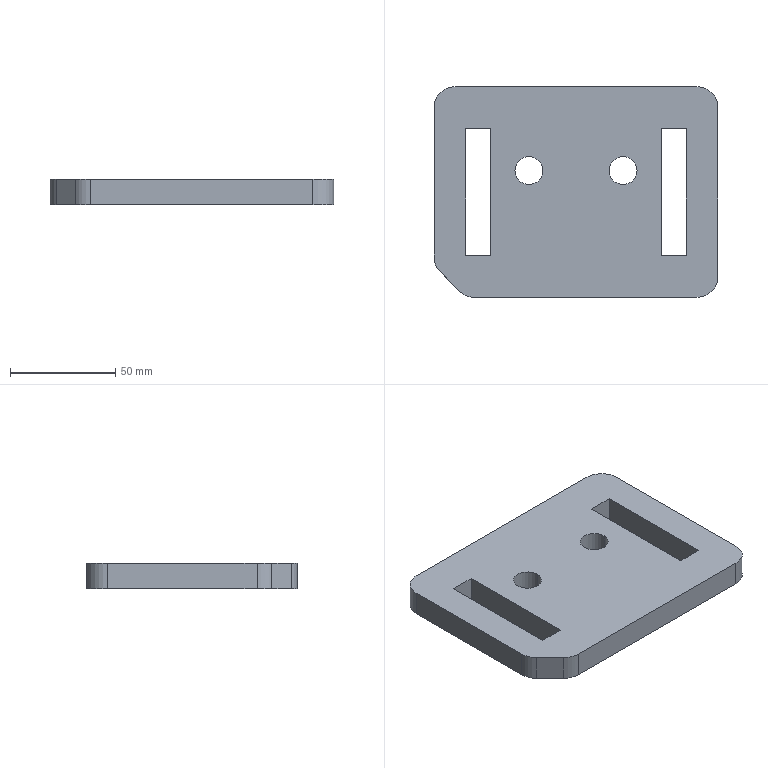Part | SolidWorks | features FlatPattern 1, SMBaseFlange 1, SheetMetal 1 | 1 solid | 24 faces | box 134.7 x 100 x 12 mm | volume 138852 mm3 | plane 15 | cylinder 9 | commonest cylinder face diameters 20 x5 13.3 x4
STEP:
#1=CARTESIAN_POINT('',(105.804,88.65,12.));
#2=VERTEX_POINT('',#1);
#3=CARTESIAN_POINT('',(119.104,88.65,12.));
#4=VERTEX_POINT('',#3);
#5=CARTESIAN_POINT('',(112.454,88.65,12.));
#6=DIRECTION('',(0.,0.,1.));
#7=DIRECTION('',(1.,0.,0.));
#8=AXIS2_PLACEMENT_3D('',#5,#6,#7);
#9=CIRCLE('',#8,6.65);
#10=EDGE_CURVE('',#2,#4,#9,.T.);
#11=ORIENTED_EDGE('',*,*,#10,.T.);
#12=CARTESIAN_POINT('',(119.104,88.65,0.));
#13=VERTEX_POINT('',#12);
#14=CARTESIAN_POINT('',(119.104,88.65,12.));
#15=DIRECTION('',(0.,0.,-1.));
#16=VECTOR('',#15,1000.);
#17=LINE('',#14,#16);
#18=EDGE_CURVE('',#4,#13,#17,.T.);
#19=ORIENTED_EDGE('',*,*,#18,.T.);
#20=CARTESIAN_POINT('',(105.804,88.65,0.));
#21=VERTEX_POINT('',#20);
#22=CARTESIAN_POINT('',(112.454,88.65,0.));
#23=DIRECTION('',(0.,0.,1.));
#24=DIRECTION('',(1.,0.,0.));
#25=AXIS2_PLACEMENT_3D('',#22,#23,#24);
#26=CIRCLE('',#25,6.65);
#27=EDGE_CURVE('',#21,#13,#26,.T.);
#28=ORIENTED_EDGE('',*,*,#27,.F.);
#29=CARTESIAN_POINT('',(105.804,88.65,12.));
#30=DIRECTION('',(0.,0.,-1.));
#31=VECTOR('',#30,1000.);
#32=LINE('',#29,#31);
#33=EDGE_CURVE('',#2,#21,#32,.T.);
#34=ORIENTED_EDGE('',*,*,#33,.F.);
#35=EDGE_LOOP('',(#11,#19,#28,#34));
#36=FACE_OUTER_BOUND('',#35,.T.);
#37=CARTESIAN_POINT('',(112.454,88.65,12.));
#38=DIRECTION('',(0.,0.,-1.));
#39=DIRECTION('',(-1.,0.,0.));
#40=AXIS2_PLACEMENT_3D('',#37,#38,#39);
#41=CYLINDRICAL_SURFACE('',#40,6.65);
#42=ADVANCED_FACE('',(#36),#41,.F.);
#43=CARTESIAN_POINT('',(61.104,88.65,12.));
#44=VERTEX_POINT('',#43);
#45=CARTESIAN_POINT('',(74.404,88.65,12.));
#46=VERTEX_POINT('',#45);
#47=CARTESIAN_POINT('',(67.754,88.65,12.));
#48=DIRECTION('',(0.,0.,1.));
#49=DIRECTION('',(1.,0.,0.));
#50=AXIS2_PLACEMENT_3D('',#47,#48,#49);
#51=CIRCLE('',#50,6.65);
#52=EDGE_CURVE('',#44,#46,#51,.T.);
#53=ORIENTED_EDGE('',*,*,#52,.T.);
#54=CARTESIAN_POINT('',(74.404,88.65,0.));
#55=VERTEX_POINT('',#54);
#56=CARTESIAN_POINT('',(74.404,88.65,12.));
#57=DIRECTION('',(0.,0.,-1.));
#58=VECTOR('',#57,1000.);
#59=LINE('',#56,#58);
#60=EDGE_CURVE('',#46,#55,#59,.T.);
#61=ORIENTED_EDGE('',*,*,#60,.T.);
#62=CARTESIAN_POINT('',(61.104,88.65,0.));
#63=VERTEX_POINT('',#62);
#64=CARTESIAN_POINT('',(67.754,88.65,0.));
#65=DIRECTION('',(0.,0.,1.));
#66=DIRECTION('',(1.,0.,0.));
#67=AXIS2_PLACEMENT_3D('',#64,#65,#66);
#68=CIRCLE('',#67,6.65);
#69=EDGE_CURVE('',#63,#55,#68,.T.);
#70=ORIENTED_EDGE('',*,*,#69,.F.);
#71=CARTESIAN_POINT('',(61.104,88.65,12.));
#72=DIRECTION('',(0.,0.,-1.));
#73=VECTOR('',#72,1000.);
#74=LINE('',#71,#73);
#75=EDGE_CURVE('',#44,#63,#74,.T.);
#76=ORIENTED_EDGE('',*,*,#75,.F.);
#77=EDGE_LOOP('',(#53,#61,#70,#76));
#78=FACE_OUTER_BOUND('',#77,.T.);
#79=CARTESIAN_POINT('',(67.754,88.65,12.));
#80=DIRECTION('',(0.,0.,-1.));
#81=DIRECTION('',(-1.,0.,0.));
#82=AXIS2_PLACEMENT_3D('',#79,#80,#81);
#83=CYLINDRICAL_SURFACE('',#82,6.65);
#84=ADVANCED_FACE('',(#78),#83,.F.);
#85=ORIENTED_EDGE('',*,*,#52,.F.);
#86=CARTESIAN_POINT('',(67.754,88.65,12.));
#87=DIRECTION('',(0.,0.,1.));
#88=DIRECTION('',(1.,0.,0.));
#89=AXIS2_PLACEMENT_3D('',#86,#87,#88);
#90=CIRCLE('',#89,6.65);
#91=EDGE_CURVE('',#46,#44,#90,.T.);
#92=ORIENTED_EDGE('',*,*,#91,.F.);
#93=EDGE_LOOP('',(#85,#92));
#94=FACE_BOUND('',#93,.T.);
#95=CARTESIAN_POINT('',(22.754,47.642,12.));
#96=VERTEX_POINT('',#95);
#97=CARTESIAN_POINT('',(25.683,40.571,12.));
#98=VERTEX_POINT('',#97);
#99=CARTESIAN_POINT('',(32.754,47.642,12.));
#100=DIRECTION('',(0.,0.,1.));
#101=DIRECTION('',(1.,0.,0.));
#102=AXIS2_PLACEMENT_3D('',#99,#100,#101);
#103=CIRCLE('',#102,10.);
#104=EDGE_CURVE('',#96,#98,#103,.T.);
#105=ORIENTED_EDGE('',*,*,#104,.T.);
#106=CARTESIAN_POINT('',(34.825,31.429,12.));
#107=VERTEX_POINT('',#106);
#108=CARTESIAN_POINT('',(34.825,31.429,12.));
#109=DIRECTION('',(0.7071,-0.7071,0.));
#110=VECTOR('',#109,1000.);
#111=LINE('',#108,#110);
#112=EDGE_CURVE('',#98,#107,#111,.T.);
#113=ORIENTED_EDGE('',*,*,#112,.T.);
#114=CARTESIAN_POINT('',(41.896,28.5,12.));
#115=VERTEX_POINT('',#114);
#116=CARTESIAN_POINT('',(41.896,38.5,12.));
#117=DIRECTION('',(0.,0.,1.));
#118=DIRECTION('',(-1.,0.,0.));
#119=AXIS2_PLACEMENT_3D('',#116,#117,#118);
#120=CIRCLE('',#119,10.);
#121=EDGE_CURVE('',#107,#115,#120,.T.);
#122=ORIENTED_EDGE('',*,*,#121,.T.);
#123=CARTESIAN_POINT('',(147.454,28.5,12.));
#124=VERTEX_POINT('',#123);
#125=CARTESIAN_POINT('',(41.896,28.5,12.));
#126=DIRECTION('',(1.,0.,0.));
#127=VECTOR('',#126,1000.);
#128=LINE('',#125,#127);
#129=EDGE_CURVE('',#115,#124,#128,.T.);
#130=ORIENTED_EDGE('',*,*,#129,.T.);
#131=CARTESIAN_POINT('',(157.454,38.5,12.));
#132=VERTEX_POINT('',#131);
#133=CARTESIAN_POINT('',(147.454,38.5,12.));
#134=DIRECTION('',(0.,0.,1.));
#135=DIRECTION('',(1.,0.,0.));
#136=AXIS2_PLACEMENT_3D('',#133,#134,#135);
#137=CIRCLE('',#136,10.);
#138=EDGE_CURVE('',#124,#132,#137,.T.);
#139=ORIENTED_EDGE('',*,*,#138,.T.);
#140=CARTESIAN_POINT('',(157.454,118.5,12.));
#141=VERTEX_POINT('',#140);
#142=CARTESIAN_POINT('',(157.454,118.5,12.));
#143=DIRECTION('',(0.,1.,0.));
#144=VECTOR('',#143,1000.);
#145=LINE('',#142,#144);
#146=EDGE_CURVE('',#132,#141,#145,.T.);
#147=ORIENTED_EDGE('',*,*,#146,.T.);
#148=CARTESIAN_POINT('',(147.454,128.5,12.));
#149=VERTEX_POINT('',#148);
#150=CARTESIAN_POINT('',(147.454,118.5,12.));
#151=DIRECTION('',(0.,0.,1.));
#152=DIRECTION('',(-1.,0.,0.));
#153=AXIS2_PLACEMENT_3D('',#150,#151,#152);
#154=CIRCLE('',#153,10.);
#155=EDGE_CURVE('',#141,#149,#154,.T.);
#156=ORIENTED_EDGE('',*,*,#155,.T.);
#157=CARTESIAN_POINT('',(32.754,128.5,12.));
#158=VERTEX_POINT('',#157);
#159=CARTESIAN_POINT('',(32.754,128.5,12.));
#160=DIRECTION('',(-1.,0.,0.));
#161=VECTOR('',#160,1000.);
#162=LINE('',#159,#161);
#163=EDGE_CURVE('',#149,#158,#162,.T.);
#164=ORIENTED_EDGE('',*,*,#163,.T.);
#165=CARTESIAN_POINT('',(22.754,118.5,12.));
#166=VERTEX_POINT('',#165);
#167=CARTESIAN_POINT('',(32.754,118.5,12.));
#168=DIRECTION('',(0.,0.,1.));
#169=DIRECTION('',(1.,0.,0.));
#170=AXIS2_PLACEMENT_3D('',#167,#168,#169);
#171=CIRCLE('',#170,10.);
#172=EDGE_CURVE('',#158,#166,#171,.T.);
#173=ORIENTED_EDGE('',*,*,#172,.T.);
#174=CARTESIAN_POINT('',(22.754,118.5,12.));
#175=DIRECTION('',(0.,-1.,0.));
#176=VECTOR('',#175,1000.);
#177=LINE('',#174,#176);
#178=EDGE_CURVE('',#166,#96,#177,.T.);
#179=ORIENTED_EDGE('',*,*,#178,.T.);
#180=EDGE_LOOP('',(#105,#113,#122,#130,#139,#147,#156,#164,#173,#179));
#181=FACE_OUTER_BOUND('',#180,.T.);
#182=ORIENTED_EDGE('',*,*,#10,.F.);
#183=CARTESIAN_POINT('',(112.454,88.65,12.));
#184=DIRECTION('',(0.,0.,1.));
#185=DIRECTION('',(1.,0.,0.));
#186=AXIS2_PLACEMENT_3D('',#183,#184,#185);
#187=CIRCLE('',#186,6.65);
#188=EDGE_CURVE('',#4,#2,#187,.T.);
#189=ORIENTED_EDGE('',*,*,#188,.F.);
#190=EDGE_LOOP('',(#182,#189));
#191=FACE_BOUND('',#190,.T.);
#192=CARTESIAN_POINT('',(142.454,108.5,12.));
#193=VERTEX_POINT('',#192);
#194=CARTESIAN_POINT('',(130.454,108.5,12.));
#195=VERTEX_POINT('',#194);
#196=CARTESIAN_POINT('',(142.454,108.5,12.));
#197=DIRECTION('',(-1.,0.,0.));
#198=VECTOR('',#197,1000.);
#199=LINE('',#196,#198);
#200=EDGE_CURVE('',#193,#195,#199,.T.);
#201=ORIENTED_EDGE('',*,*,#200,.F.);
#202=CARTESIAN_POINT('',(142.454,48.5,12.));
#203=VERTEX_POINT('',#202);
#204=CARTESIAN_POINT('',(142.454,108.5,12.));
#205=DIRECTION('',(0.,1.,0.));
#206=VECTOR('',#205,1000.);
#207=LINE('',#204,#206);
#208=EDGE_CURVE('',#203,#193,#207,.T.);
#209=ORIENTED_EDGE('',*,*,#208,.F.);
#210=CARTESIAN_POINT('',(130.454,48.5,12.));
#211=VERTEX_POINT('',#210);
#212=CARTESIAN_POINT('',(142.454,48.5,12.));
#213=DIRECTION('',(1.,0.,0.));
#214=VECTOR('',#213,1000.);
#215=LINE('',#212,#214);
#216=EDGE_CURVE('',#211,#203,#215,.T.);
#217=ORIENTED_EDGE('',*,*,#216,.F.);
#218=CARTESIAN_POINT('',(130.454,108.5,12.));
#219=DIRECTION('',(0.,-1.,0.));
#220=VECTOR('',#219,1000.);
#221=LINE('',#218,#220);
#222=EDGE_CURVE('',#195,#211,#221,.T.);
#223=ORIENTED_EDGE('',*,*,#222,.F.);
#224=EDGE_LOOP('',(#201,#209,#217,#223));
#225=FACE_BOUND('',#224,.T.);
#226=CARTESIAN_POINT('',(49.754,108.5,12.));
#227=VERTEX_POINT('',#226);
#228=CARTESIAN_POINT('',(37.754,108.5,12.));
#229=VERTEX_POINT('',#228);
#230=CARTESIAN_POINT('',(49.754,108.5,12.));
#231=DIRECTION('',(-1.,0.,0.));
#232=VECTOR('',#231,1000.);
#233=LINE('',#230,#232);
#234=EDGE_CURVE('',#227,#229,#233,.T.);
#235=ORIENTED_EDGE('',*,*,#234,.F.);
#236=CARTESIAN_POINT('',(49.754,48.5,12.));
#237=VERTEX_POINT('',#236);
#238=CARTESIAN_POINT('',(49.754,108.5,12.));
#239=DIRECTION('',(0.,1.,0.));
#240=VECTOR('',#239,1000.);
#241=LINE('',#238,#240);
#242=EDGE_CURVE('',#237,#227,#241,.T.);
#243=ORIENTED_EDGE('',*,*,#242,.F.);
#244=CARTESIAN_POINT('',(37.754,48.5,12.));
#245=VERTEX_POINT('',#244);
#246=CARTESIAN_POINT('',(49.754,48.5,12.));
#247=DIRECTION('',(1.,0.,0.));
#248=VECTOR('',#247,1000.);
#249=LINE('',#246,#248);
#250=EDGE_CURVE('',#245,#237,#249,.T.);
#251=ORIENTED_EDGE('',*,*,#250,.F.);
#252=CARTESIAN_POINT('',(37.754,108.5,12.));
#253=DIRECTION('',(0.,-1.,0.));
#254=VECTOR('',#253,1000.);
#255=LINE('',#252,#254);
#256=EDGE_CURVE('',#229,#245,#255,.T.);
#257=ORIENTED_EDGE('',*,*,#256,.F.);
#258=EDGE_LOOP('',(#235,#243,#251,#257));
#259=FACE_BOUND('',#258,.T.);
#260=CARTESIAN_POINT('',(32.754,47.642,12.));
#261=DIRECTION('',(0.,0.,1.));
#262=DIRECTION('',(1.,0.,0.));
#263=AXIS2_PLACEMENT_3D('',#260,#261,#262);
#264=PLANE('',#263);
#265=ADVANCED_FACE('',(#94,#181,#191,#225,#259),#264,.T.);
#266=CARTESIAN_POINT('',(142.454,48.5,0.));
#267=VERTEX_POINT('',#266);
#268=CARTESIAN_POINT('',(142.454,108.5,0.));
#269=VERTEX_POINT('',#268);
#270=CARTESIAN_POINT('',(142.454,108.5,0.));
#271=DIRECTION('',(0.,1.,0.));
#272=VECTOR('',#271,1000.);
#273=LINE('',#270,#272);
#274=EDGE_CURVE('',#267,#269,#273,.T.);
#275=ORIENTED_EDGE('',*,*,#274,.T.);
#276=CARTESIAN_POINT('',(130.454,108.5,0.));
#277=VERTEX_POINT('',#276);
#278=CARTESIAN_POINT('',(142.454,108.5,0.));
#279=DIRECTION('',(-1.,0.,0.));
#280=VECTOR('',#279,1000.);
#281=LINE('',#278,#280);
#282=EDGE_CURVE('',#269,#277,#281,.T.);
#283=ORIENTED_EDGE('',*,*,#282,.T.);
#284=CARTESIAN_POINT('',(130.454,48.5,0.));
#285=VERTEX_POINT('',#284);
#286=CARTESIAN_POINT('',(130.454,108.5,0.));
#287=DIRECTION('',(0.,-1.,0.));
#288=VECTOR('',#287,1000.);
#289=LINE('',#286,#288);
#290=EDGE_CURVE('',#277,#285,#289,.T.);
#291=ORIENTED_EDGE('',*,*,#290,.T.);
#292=CARTESIAN_POINT('',(142.454,48.5,0.));
#293=DIRECTION('',(1.,0.,0.));
#294=VECTOR('',#293,1000.);
#295=LINE('',#292,#294);
#296=EDGE_CURVE('',#285,#267,#295,.T.);
#297=ORIENTED_EDGE('',*,*,#296,.T.);
#298=EDGE_LOOP('',(#275,#283,#291,#297));
#299=FACE_BOUND('',#298,.T.);
#300=CARTESIAN_POINT('',(22.754,47.642,0.));
#301=VERTEX_POINT('',#300);
#302=CARTESIAN_POINT('',(25.683,40.571,0.));
#303=VERTEX_POINT('',#302);
#304=CARTESIAN_POINT('',(32.754,47.642,0.));
#305=DIRECTION('',(0.,0.,1.));
#306=DIRECTION('',(1.,0.,0.));
#307=AXIS2_PLACEMENT_3D('',#304,#305,#306);
#308=CIRCLE('',#307,10.);
#309=EDGE_CURVE('',#301,#303,#308,.T.);
#310=ORIENTED_EDGE('',*,*,#309,.F.);
#311=CARTESIAN_POINT('',(22.754,118.5,0.));
#312=VERTEX_POINT('',#311);
#313=CARTESIAN_POINT('',(22.754,118.5,0.));
#314=DIRECTION('',(0.,-1.,0.));
#315=VECTOR('',#314,1000.);
#316=LINE('',#313,#315);
#317=EDGE_CURVE('',#312,#301,#316,.T.);
#318=ORIENTED_EDGE('',*,*,#317,.F.);
#319=CARTESIAN_POINT('',(32.754,128.5,0.));
#320=VERTEX_POINT('',#319);
#321=CARTESIAN_POINT('',(32.754,118.5,0.));
#322=DIRECTION('',(0.,0.,1.));
#323=DIRECTION('',(1.,0.,0.));
#324=AXIS2_PLACEMENT_3D('',#321,#322,#323);
#325=CIRCLE('',#324,10.);
#326=EDGE_CURVE('',#320,#312,#325,.T.);
#327=ORIENTED_EDGE('',*,*,#326,.F.);
#328=CARTESIAN_POINT('',(147.454,128.5,0.));
#329=VERTEX_POINT('',#328);
#330=CARTESIAN_POINT('',(32.754,128.5,0.));
#331=DIRECTION('',(-1.,0.,0.));
#332=VECTOR('',#331,1000.);
#333=LINE('',#330,#332);
#334=EDGE_CURVE('',#329,#320,#333,.T.);
#335=ORIENTED_EDGE('',*,*,#334,.F.);
#336=CARTESIAN_POINT('',(157.454,118.5,0.));
#337=VERTEX_POINT('',#336);
#338=CARTESIAN_POINT('',(147.454,118.5,0.));
#339=DIRECTION('',(0.,0.,1.));
#340=DIRECTION('',(-1.,0.,0.));
#341=AXIS2_PLACEMENT_3D('',#338,#339,#340);
#342=CIRCLE('',#341,10.);
#343=EDGE_CURVE('',#337,#329,#342,.T.);
#344=ORIENTED_EDGE('',*,*,#343,.F.);
#345=CARTESIAN_POINT('',(157.454,38.5,0.));
#346=VERTEX_POINT('',#345);
#347=CARTESIAN_POINT('',(157.454,118.5,0.));
#348=DIRECTION('',(0.,1.,0.));
#349=VECTOR('',#348,1000.);
#350=LINE('',#347,#349);
#351=EDGE_CURVE('',#346,#337,#350,.T.);
#352=ORIENTED_EDGE('',*,*,#351,.F.);
#353=CARTESIAN_POINT('',(147.454,28.5,0.));
#354=VERTEX_POINT('',#353);
#355=CARTESIAN_POINT('',(147.454,38.5,0.));
#356=DIRECTION('',(0.,0.,1.));
#357=DIRECTION('',(1.,0.,0.));
#358=AXIS2_PLACEMENT_3D('',#355,#356,#357);
#359=CIRCLE('',#358,10.);
#360=EDGE_CURVE('',#354,#346,#359,.T.);
#361=ORIENTED_EDGE('',*,*,#360,.F.);
#362=CARTESIAN_POINT('',(41.896,28.5,0.));
#363=VERTEX_POINT('',#362);
#364=CARTESIAN_POINT('',(41.896,28.5,0.));
#365=DIRECTION('',(1.,0.,0.));
#366=VECTOR('',#365,1000.);
#367=LINE('',#364,#366);
#368=EDGE_CURVE('',#363,#354,#367,.T.);
#369=ORIENTED_EDGE('',*,*,#368,.F.);
#370=CARTESIAN_POINT('',(34.825,31.429,0.));
#371=VERTEX_POINT('',#370);
#372=CARTESIAN_POINT('',(41.896,38.5,0.));
#373=DIRECTION('',(0.,0.,1.));
#374=DIRECTION('',(-1.,0.,0.));
#375=AXIS2_PLACEMENT_3D('',#372,#373,#374);
#376=CIRCLE('',#375,10.);
#377=EDGE_CURVE('',#371,#363,#376,.T.);
#378=ORIENTED_EDGE('',*,*,#377,.F.);
#379=CARTESIAN_POINT('',(34.825,31.429,0.));
#380=DIRECTION('',(0.7071,-0.7071,0.));
#381=VECTOR('',#380,1000.);
#382=LINE('',#379,#381);
#383=EDGE_CURVE('',#303,#371,#382,.T.);
#384=ORIENTED_EDGE('',*,*,#383,.F.);
#385=EDGE_LOOP('',(#310,#318,#327,#335,#344,#352,#361,#369,#378,#384));
#386=FACE_OUTER_BOUND('',#385,.T.);
#387=ORIENTED_EDGE('',*,*,#69,.T.);
#388=CARTESIAN_POINT('',(67.754,88.65,0.));
#389=DIRECTION('',(0.,0.,1.));
#390=DIRECTION('',(1.,0.,0.));
#391=AXIS2_PLACEMENT_3D('',#388,#389,#390);
#392=CIRCLE('',#391,6.65);
#393=EDGE_CURVE('',#55,#63,#392,.T.);
#394=ORIENTED_EDGE('',*,*,#393,.T.);
#395=EDGE_LOOP('',(#387,#394));
#396=FACE_BOUND('',#395,.T.);
#397=ORIENTED_EDGE('',*,*,#27,.T.);
#398=CARTESIAN_POINT('',(112.454,88.65,0.));
#399=DIRECTION('',(0.,0.,1.));
#400=DIRECTION('',(1.,0.,0.));
#401=AXIS2_PLACEMENT_3D('',#398,#399,#400);
#402=CIRCLE('',#401,6.65);
#403=EDGE_CURVE('',#13,#21,#402,.T.);
#404=ORIENTED_EDGE('',*,*,#403,.T.);
#405=EDGE_LOOP('',(#397,#404));
#406=FACE_BOUND('',#405,.T.);
#407=CARTESIAN_POINT('',(49.754,48.5,0.));
#408=VERTEX_POINT('',#407);
#409=CARTESIAN_POINT('',(49.754,108.5,0.));
#410=VERTEX_POINT('',#409);
#411=CARTESIAN_POINT('',(49.754,108.5,0.));
#412=DIRECTION('',(0.,1.,0.));
#413=VECTOR('',#412,1000.);
#414=LINE('',#411,#413);
#415=EDGE_CURVE('',#408,#410,#414,.T.);
#416=ORIENTED_EDGE('',*,*,#415,.T.);
#417=CARTESIAN_POINT('',(37.754,108.5,0.));
#418=VERTEX_POINT('',#417);
#419=CARTESIAN_POINT('',(49.754,108.5,0.));
#420=DIRECTION('',(-1.,0.,0.));
#421=VECTOR('',#420,1000.);
#422=LINE('',#419,#421);
#423=EDGE_CURVE('',#410,#418,#422,.T.);
#424=ORIENTED_EDGE('',*,*,#423,.T.);
#425=CARTESIAN_POINT('',(37.754,48.5,0.));
#426=VERTEX_POINT('',#425);
#427=CARTESIAN_POINT('',(37.754,108.5,0.));
#428=DIRECTION('',(0.,-1.,0.));
#429=VECTOR('',#428,1000.);
#430=LINE('',#427,#429);
#431=EDGE_CURVE('',#418,#426,#430,.T.);
#432=ORIENTED_EDGE('',*,*,#431,.T.);
#433=CARTESIAN_POINT('',(49.754,48.5,0.));
#434=DIRECTION('',(1.,0.,0.));
#435=VECTOR('',#434,1000.);
#436=LINE('',#433,#435);
#437=EDGE_CURVE('',#426,#408,#436,.T.);
#438=ORIENTED_EDGE('',*,*,#437,.T.);
#439=EDGE_LOOP('',(#416,#424,#432,#438));
#440=FACE_BOUND('',#439,.T.);
#441=CARTESIAN_POINT('',(32.754,47.642,0.));
#442=DIRECTION('',(0.,0.,1.));
#443=DIRECTION('',(1.,0.,0.));
#444=AXIS2_PLACEMENT_3D('',#441,#442,#443);
#445=PLANE('',#444);
#446=ADVANCED_FACE('',(#299,#386,#396,#406,#440),#445,.F.);
#447=ORIENTED_EDGE('',*,*,#309,.T.);
#448=CARTESIAN_POINT('',(25.683,40.571,12.));
#449=DIRECTION('',(0.,0.,-1.));
#450=VECTOR('',#449,1000.);
#451=LINE('',#448,#450);
#452=EDGE_CURVE('',#98,#303,#451,.T.);
#453=ORIENTED_EDGE('',*,*,#452,.F.);
#454=ORIENTED_EDGE('',*,*,#104,.F.);
#455=CARTESIAN_POINT('',(22.754,47.642,12.));
#456=DIRECTION('',(0.,0.,-1.));
#457=VECTOR('',#456,1000.);
#458=LINE('',#455,#457);
#459=EDGE_CURVE('',#96,#301,#458,.T.);
#460=ORIENTED_EDGE('',*,*,#459,.T.);
#461=EDGE_LOOP('',(#447,#453,#454,#460));
#462=FACE_OUTER_BOUND('',#461,.T.);
#463=CARTESIAN_POINT('',(32.754,47.642,12.));
#464=DIRECTION('',(0.,0.,-1.));
#465=DIRECTION('',(-1.,0.,0.));
#466=AXIS2_PLACEMENT_3D('',#463,#464,#465);
#467=CYLINDRICAL_SURFACE('',#466,10.);
#468=ADVANCED_FACE('',(#462),#467,.T.);
#469=ORIENTED_EDGE('',*,*,#383,.T.);
#470=CARTESIAN_POINT('',(34.825,31.429,12.));
#471=DIRECTION('',(0.,0.,-1.));
#472=VECTOR('',#471,1000.);
#473=LINE('',#470,#472);
#474=EDGE_CURVE('',#107,#371,#473,.T.);
#475=ORIENTED_EDGE('',*,*,#474,.F.);
#476=ORIENTED_EDGE('',*,*,#112,.F.);
#477=ORIENTED_EDGE('',*,*,#452,.T.);
#478=EDGE_LOOP('',(#469,#475,#476,#477));
#479=FACE_OUTER_BOUND('',#478,.T.);
#480=CARTESIAN_POINT('',(34.825,31.429,12.));
#481=DIRECTION('',(0.7071,0.7071,0.));
#482=DIRECTION('',(-0.7071,0.7071,0.));
#483=AXIS2_PLACEMENT_3D('',#480,#481,#482);
#484=PLANE('',#483);
#485=ADVANCED_FACE('',(#479),#484,.F.);
#486=ORIENTED_EDGE('',*,*,#377,.T.);
#487=CARTESIAN_POINT('',(41.896,28.5,12.));
#488=DIRECTION('',(0.,0.,-1.));
#489=VECTOR('',#488,1000.);
#490=LINE('',#487,#489);
#491=EDGE_CURVE('',#115,#363,#490,.T.);
#492=ORIENTED_EDGE('',*,*,#491,.F.);
#493=ORIENTED_EDGE('',*,*,#121,.F.);
#494=ORIENTED_EDGE('',*,*,#474,.T.);
#495=EDGE_LOOP('',(#486,#492,#493,#494));
#496=FACE_OUTER_BOUND('',#495,.T.);
#497=CARTESIAN_POINT('',(41.896,38.5,12.));
#498=DIRECTION('',(0.,0.,-1.));
#499=DIRECTION('',(-1.,0.,0.));
#500=AXIS2_PLACEMENT_3D('',#497,#498,#499);
#501=CYLINDRICAL_SURFACE('',#500,10.);
#502=ADVANCED_FACE('',(#496),#501,.T.);
#503=ORIENTED_EDGE('',*,*,#368,.T.);
#504=CARTESIAN_POINT('',(147.454,28.5,12.));
#505=DIRECTION('',(0.,0.,-1.));
#506=VECTOR('',#505,1000.);
#507=LINE('',#504,#506);
#508=EDGE_CURVE('',#124,#354,#507,.T.);
#509=ORIENTED_EDGE('',*,*,#508,.F.);
#510=ORIENTED_EDGE('',*,*,#129,.F.);
#511=ORIENTED_EDGE('',*,*,#491,.T.);
#512=EDGE_LOOP('',(#503,#509,#510,#511));
#513=FACE_OUTER_BOUND('',#512,.T.);
#514=CARTESIAN_POINT('',(41.896,28.5,12.));
#515=DIRECTION('',(0.,1.,0.));
#516=DIRECTION('',(-1.,0.,0.));
#517=AXIS2_PLACEMENT_3D('',#514,#515,#516);
#518=PLANE('',#517);
#519=ADVANCED_FACE('',(#513),#518,.F.);
#520=ORIENTED_EDGE('',*,*,#360,.T.);
#521=CARTESIAN_POINT('',(157.454,38.5,12.));
#522=DIRECTION('',(0.,0.,-1.));
#523=VECTOR('',#522,1000.);
#524=LINE('',#521,#523);
#525=EDGE_CURVE('',#132,#346,#524,.T.);
#526=ORIENTED_EDGE('',*,*,#525,.F.);
#527=ORIENTED_EDGE('',*,*,#138,.F.);
#528=ORIENTED_EDGE('',*,*,#508,.T.);
#529=EDGE_LOOP('',(#520,#526,#527,#528));
#530=FACE_OUTER_BOUND('',#529,.T.);
#531=CARTESIAN_POINT('',(147.454,38.5,12.));
#532=DIRECTION('',(0.,0.,-1.));
#533=DIRECTION('',(-1.,0.,0.));
#534=AXIS2_PLACEMENT_3D('',#531,#532,#533);
#535=CYLINDRICAL_SURFACE('',#534,10.);
#536=ADVANCED_FACE('',(#530),#535,.T.);
#537=ORIENTED_EDGE('',*,*,#351,.T.);
#538=CARTESIAN_POINT('',(157.454,118.5,12.));
#539=DIRECTION('',(0.,0.,-1.));
#540=VECTOR('',#539,1000.);
#541=LINE('',#538,#540);
#542=EDGE_CURVE('',#141,#337,#541,.T.);
#543=ORIENTED_EDGE('',*,*,#542,.F.);
#544=ORIENTED_EDGE('',*,*,#146,.F.);
#545=ORIENTED_EDGE('',*,*,#525,.T.);
#546=EDGE_LOOP('',(#537,#543,#544,#545));
#547=FACE_OUTER_BOUND('',#546,.T.);
#548=CARTESIAN_POINT('',(157.454,118.5,12.));
#549=DIRECTION('',(-1.,0.,0.));
#550=DIRECTION('',(0.,0.,1.));
#551=AXIS2_PLACEMENT_3D('',#548,#549,#550);
#552=PLANE('',#551);
#553=ADVANCED_FACE('',(#547),#552,.F.);
#554=ORIENTED_EDGE('',*,*,#343,.T.);
#555=CARTESIAN_POINT('',(147.454,128.5,12.));
#556=DIRECTION('',(0.,0.,-1.));
#557=VECTOR('',#556,1000.);
#558=LINE('',#555,#557);
#559=EDGE_CURVE('',#149,#329,#558,.T.);
#560=ORIENTED_EDGE('',*,*,#559,.F.);
#561=ORIENTED_EDGE('',*,*,#155,.F.);
#562=ORIENTED_EDGE('',*,*,#542,.T.);
#563=EDGE_LOOP('',(#554,#560,#561,#562));
#564=FACE_OUTER_BOUND('',#563,.T.);
#565=CARTESIAN_POINT('',(147.454,118.5,12.));
#566=DIRECTION('',(0.,0.,-1.));
#567=DIRECTION('',(-1.,0.,0.));
#568=AXIS2_PLACEMENT_3D('',#565,#566,#567);
#569=CYLINDRICAL_SURFACE('',#568,10.);
#570=ADVANCED_FACE('',(#564),#569,.T.);
#571=ORIENTED_EDGE('',*,*,#334,.T.);
#572=CARTESIAN_POINT('',(32.754,128.5,12.));
#573=DIRECTION('',(0.,0.,-1.));
#574=VECTOR('',#573,1000.);
#575=LINE('',#572,#574);
#576=EDGE_CURVE('',#158,#320,#575,.T.);
#577=ORIENTED_EDGE('',*,*,#576,.F.);
#578=ORIENTED_EDGE('',*,*,#163,.F.);
#579=ORIENTED_EDGE('',*,*,#559,.T.);
#580=EDGE_LOOP('',(#571,#577,#578,#579));
#581=FACE_OUTER_BOUND('',#580,.T.);
#582=CARTESIAN_POINT('',(32.754,128.5,12.));
#583=DIRECTION('',(0.,-1.,0.));
#584=DIRECTION('',(0.,0.,-1.));
#585=AXIS2_PLACEMENT_3D('',#582,#583,#584);
#586=PLANE('',#585);
#587=ADVANCED_FACE('',(#581),#586,.F.);
#588=ORIENTED_EDGE('',*,*,#326,.T.);
#589=CARTESIAN_POINT('',(22.754,118.5,12.));
#590=DIRECTION('',(0.,0.,-1.));
#591=VECTOR('',#590,1000.);
#592=LINE('',#589,#591);
#593=EDGE_CURVE('',#166,#312,#592,.T.);
#594=ORIENTED_EDGE('',*,*,#593,.F.);
#595=ORIENTED_EDGE('',*,*,#172,.F.);
#596=ORIENTED_EDGE('',*,*,#576,.T.);
#597=EDGE_LOOP('',(#588,#594,#595,#596));
#598=FACE_OUTER_BOUND('',#597,.T.);
#599=CARTESIAN_POINT('',(32.754,118.5,12.));
#600=DIRECTION('',(0.,0.,-1.));
#601=DIRECTION('',(-1.,0.,0.));
#602=AXIS2_PLACEMENT_3D('',#599,#600,#601);
#603=CYLINDRICAL_SURFACE('',#602,10.);
#604=ADVANCED_FACE('',(#598),#603,.T.);
#605=ORIENTED_EDGE('',*,*,#317,.T.);
#606=ORIENTED_EDGE('',*,*,#459,.F.);
#607=ORIENTED_EDGE('',*,*,#178,.F.);
#608=ORIENTED_EDGE('',*,*,#593,.T.);
#609=EDGE_LOOP('',(#605,#606,#607,#608));
#610=FACE_OUTER_BOUND('',#609,.T.);
#611=CARTESIAN_POINT('',(22.754,118.5,12.));
#612=DIRECTION('',(1.,0.,0.));
#613=DIRECTION('',(0.,1.,0.));
#614=AXIS2_PLACEMENT_3D('',#611,#612,#613);
#615=PLANE('',#614);
#616=ADVANCED_FACE('',(#610),#615,.F.);
#617=ORIENTED_EDGE('',*,*,#60,.F.);
#618=ORIENTED_EDGE('',*,*,#91,.T.);
#619=ORIENTED_EDGE('',*,*,#75,.T.);
#620=ORIENTED_EDGE('',*,*,#393,.F.);
#621=EDGE_LOOP('',(#617,#618,#619,#620));
#622=FACE_OUTER_BOUND('',#621,.T.);
#623=CARTESIAN_POINT('',(67.754,88.65,12.));
#624=DIRECTION('',(0.,0.,-1.));
#625=DIRECTION('',(-1.,0.,0.));
#626=AXIS2_PLACEMENT_3D('',#623,#624,#625);
#627=CYLINDRICAL_SURFACE('',#626,6.65);
#628=ADVANCED_FACE('',(#622),#627,.F.);
#629=ORIENTED_EDGE('',*,*,#18,.F.);
#630=ORIENTED_EDGE('',*,*,#188,.T.);
#631=ORIENTED_EDGE('',*,*,#33,.T.);
#632=ORIENTED_EDGE('',*,*,#403,.F.);
#633=EDGE_LOOP('',(#629,#630,#631,#632));
#634=FACE_OUTER_BOUND('',#633,.T.);
#635=CARTESIAN_POINT('',(112.454,88.65,12.));
#636=DIRECTION('',(0.,0.,-1.));
#637=DIRECTION('',(-1.,0.,0.));
#638=AXIS2_PLACEMENT_3D('',#635,#636,#637);
#639=CYLINDRICAL_SURFACE('',#638,6.65);
#640=ADVANCED_FACE('',(#634),#639,.F.);
#641=ORIENTED_EDGE('',*,*,#274,.F.);
#642=CARTESIAN_POINT('',(142.454,48.5,12.));
#643=DIRECTION('',(0.,0.,-1.));
#644=VECTOR('',#643,1000.);
#645=LINE('',#642,#644);
#646=EDGE_CURVE('',#203,#267,#645,.T.);
#647=ORIENTED_EDGE('',*,*,#646,.F.);
#648=ORIENTED_EDGE('',*,*,#208,.T.);
#649=CARTESIAN_POINT('',(142.454,108.5,12.));
#650=DIRECTION('',(0.,0.,-1.));
#651=VECTOR('',#650,1000.);
#652=LINE('',#649,#651);
#653=EDGE_CURVE('',#193,#269,#652,.T.);
#654=ORIENTED_EDGE('',*,*,#653,.T.);
#655=EDGE_LOOP('',(#641,#647,#648,#654));
#656=FACE_OUTER_BOUND('',#655,.T.);
#657=CARTESIAN_POINT('',(142.454,108.5,12.));
#658=DIRECTION('',(-1.,0.,0.));
#659=DIRECTION('',(0.,0.,1.));
#660=AXIS2_PLACEMENT_3D('',#657,#658,#659);
#661=PLANE('',#660);
#662=ADVANCED_FACE('',(#656),#661,.T.);
#663=ORIENTED_EDGE('',*,*,#282,.F.);
#664=ORIENTED_EDGE('',*,*,#653,.F.);
#665=ORIENTED_EDGE('',*,*,#200,.T.);
#666=CARTESIAN_POINT('',(130.454,108.5,12.));
#667=DIRECTION('',(0.,0.,-1.));
#668=VECTOR('',#667,1000.);
#669=LINE('',#666,#668);
#670=EDGE_CURVE('',#195,#277,#669,.T.);
#671=ORIENTED_EDGE('',*,*,#670,.T.);
#672=EDGE_LOOP('',(#663,#664,#665,#671));
#673=FACE_OUTER_BOUND('',#672,.T.);
#674=CARTESIAN_POINT('',(142.454,108.5,12.));
#675=DIRECTION('',(0.,-1.,0.));
#676=DIRECTION('',(0.,0.,-1.));
#677=AXIS2_PLACEMENT_3D('',#674,#675,#676);
#678=PLANE('',#677);
#679=ADVANCED_FACE('',(#673),#678,.T.);
#680=ORIENTED_EDGE('',*,*,#290,.F.);
#681=ORIENTED_EDGE('',*,*,#670,.F.);
#682=ORIENTED_EDGE('',*,*,#222,.T.);
#683=CARTESIAN_POINT('',(130.454,48.5,12.));
#684=DIRECTION('',(0.,0.,-1.));
#685=VECTOR('',#684,1000.);
#686=LINE('',#683,#685);
#687=EDGE_CURVE('',#211,#285,#686,.T.);
#688=ORIENTED_EDGE('',*,*,#687,.T.);
#689=EDGE_LOOP('',(#680,#681,#682,#688));
#690=FACE_OUTER_BOUND('',#689,.T.);
#691=CARTESIAN_POINT('',(130.454,108.5,12.));
#692=DIRECTION('',(1.,0.,0.));
#693=DIRECTION('',(0.,0.,-1.));
#694=AXIS2_PLACEMENT_3D('',#691,#692,#693);
#695=PLANE('',#694);
#696=ADVANCED_FACE('',(#690),#695,.T.);
#697=ORIENTED_EDGE('',*,*,#296,.F.);
#698=ORIENTED_EDGE('',*,*,#687,.F.);
#699=ORIENTED_EDGE('',*,*,#216,.T.);
#700=ORIENTED_EDGE('',*,*,#646,.T.);
#701=EDGE_LOOP('',(#697,#698,#699,#700));
#702=FACE_OUTER_BOUND('',#701,.T.);
#703=CARTESIAN_POINT('',(142.454,48.5,12.));
#704=DIRECTION('',(0.,1.,0.));
#705=DIRECTION('',(-1.,0.,0.));
#706=AXIS2_PLACEMENT_3D('',#703,#704,#705);
#707=PLANE('',#706);
#708=ADVANCED_FACE('',(#702),#707,.T.);
#709=ORIENTED_EDGE('',*,*,#415,.F.);
#710=CARTESIAN_POINT('',(49.754,48.5,12.));
#711=DIRECTION('',(0.,0.,-1.));
#712=VECTOR('',#711,1000.);
#713=LINE('',#710,#712);
#714=EDGE_CURVE('',#237,#408,#713,.T.);
#715=ORIENTED_EDGE('',*,*,#714,.F.);
#716=ORIENTED_EDGE('',*,*,#242,.T.);
#717=CARTESIAN_POINT('',(49.754,108.5,12.));
#718=DIRECTION('',(0.,0.,-1.));
#719=VECTOR('',#718,1000.);
#720=LINE('',#717,#719);
#721=EDGE_CURVE('',#227,#410,#720,.T.);
#722=ORIENTED_EDGE('',*,*,#721,.T.);
#723=EDGE_LOOP('',(#709,#715,#716,#722));
#724=FACE_OUTER_BOUND('',#723,.T.);
#725=CARTESIAN_POINT('',(49.754,108.5,12.));
#726=DIRECTION('',(-1.,0.,0.));
#727=DIRECTION('',(0.,-1.,0.));
#728=AXIS2_PLACEMENT_3D('',#725,#726,#727);
#729=PLANE('',#728);
#730=ADVANCED_FACE('',(#724),#729,.T.);
#731=ORIENTED_EDGE('',*,*,#423,.F.);
#732=ORIENTED_EDGE('',*,*,#721,.F.);
#733=ORIENTED_EDGE('',*,*,#234,.T.);
#734=CARTESIAN_POINT('',(37.754,108.5,12.));
#735=DIRECTION('',(0.,0.,-1.));
#736=VECTOR('',#735,1000.);
#737=LINE('',#734,#736);
#738=EDGE_CURVE('',#229,#418,#737,.T.);
#739=ORIENTED_EDGE('',*,*,#738,.T.);
#740=EDGE_LOOP('',(#731,#732,#733,#739));
#741=FACE_OUTER_BOUND('',#740,.T.);
#742=CARTESIAN_POINT('',(49.754,108.5,12.));
#743=DIRECTION('',(0.,-1.,0.));
#744=DIRECTION('',(0.,0.,-1.));
#745=AXIS2_PLACEMENT_3D('',#742,#743,#744);
#746=PLANE('',#745);
#747=ADVANCED_FACE('',(#741),#746,.T.);
#748=ORIENTED_EDGE('',*,*,#431,.F.);
#749=ORIENTED_EDGE('',*,*,#738,.F.);
#750=ORIENTED_EDGE('',*,*,#256,.T.);
#751=CARTESIAN_POINT('',(37.754,48.5,12.));
#752=DIRECTION('',(0.,0.,-1.));
#753=VECTOR('',#752,1000.);
#754=LINE('',#751,#753);
#755=EDGE_CURVE('',#245,#426,#754,.T.);
#756=ORIENTED_EDGE('',*,*,#755,.T.);
#757=EDGE_LOOP('',(#748,#749,#750,#756));
#758=FACE_OUTER_BOUND('',#757,.T.);
#759=CARTESIAN_POINT('',(37.754,108.5,12.));
#760=DIRECTION('',(1.,0.,0.));
#761=DIRECTION('',(0.,1.,0.));
#762=AXIS2_PLACEMENT_3D('',#759,#760,#761);
#763=PLANE('',#762);
#764=ADVANCED_FACE('',(#758),#763,.T.);
#765=ORIENTED_EDGE('',*,*,#437,.F.);
#766=ORIENTED_EDGE('',*,*,#755,.F.);
#767=ORIENTED_EDGE('',*,*,#250,.T.);
#768=ORIENTED_EDGE('',*,*,#714,.T.);
#769=EDGE_LOOP('',(#765,#766,#767,#768));
#770=FACE_OUTER_BOUND('',#769,.T.);
#771=CARTESIAN_POINT('',(49.754,48.5,12.));
#772=DIRECTION('',(0.,1.,0.));
#773=DIRECTION('',(0.,0.,1.));
#774=AXIS2_PLACEMENT_3D('',#771,#772,#773);
#775=PLANE('',#774);
#776=ADVANCED_FACE('',(#770),#775,.T.);
#777=CLOSED_SHELL('',(#42,#84,#265,#446,#468,#485,#502,#519,#536,#553,#570,#587,#604,#616,#628,#640,#662,#679,#696,#708,#730,#747,#764,#776));
#778=MANIFOLD_SOLID_BREP('',#777);
#779=CARTESIAN_POINT('',(0.,0.,0.));
#780=DIRECTION('',(0.,0.,1.));
#781=DIRECTION('',(1.,0.,0.));
#782=AXIS2_PLACEMENT_3D('',#779,#780,#781);
#783=(LENGTH_UNIT()NAMED_UNIT(*)SI_UNIT(.MILLI.,.METRE.));
#784=UNCERTAINTY_MEASURE_WITH_UNIT(LENGTH_MEASURE(0.00001),#783,'','');
#785=(NAMED_UNIT(*)PLANE_ANGLE_UNIT()SI_UNIT($,.RADIAN.));
#786=(NAMED_UNIT(*)SI_UNIT($,.STERADIAN.)SOLID_ANGLE_UNIT());
#787=(GEOMETRIC_REPRESENTATION_CONTEXT(3)GLOBAL_UNCERTAINTY_ASSIGNED_CONTEXT((#784))GLOBAL_UNIT_ASSIGNED_CONTEXT((#783,#785,#786))REPRESENTATION_CONTEXT('',''));
#788=ADVANCED_BREP_SHAPE_REPRESENTATION('',(#778,#782),#787);